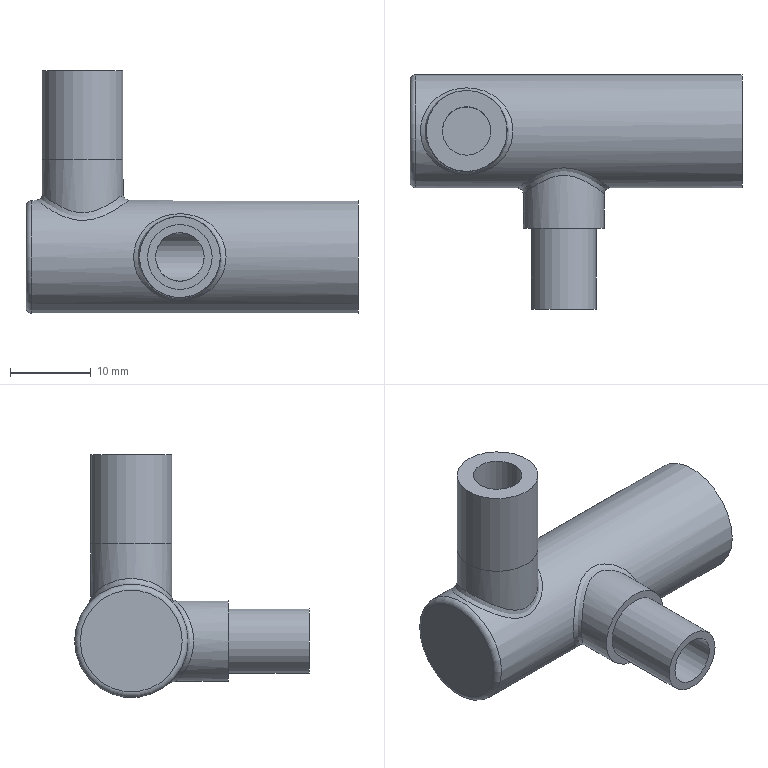Part | STEP file | 1-75.1 | 1 solid | 21 faces | box 41 x 29 x 30 mm | volume 6004 mm3 | cylinder 10 | plane 8 | spline 2 | torus 1 | commonest cylinder face diameters 6 x3 10 x3 8 x2 4 x1 14 x1